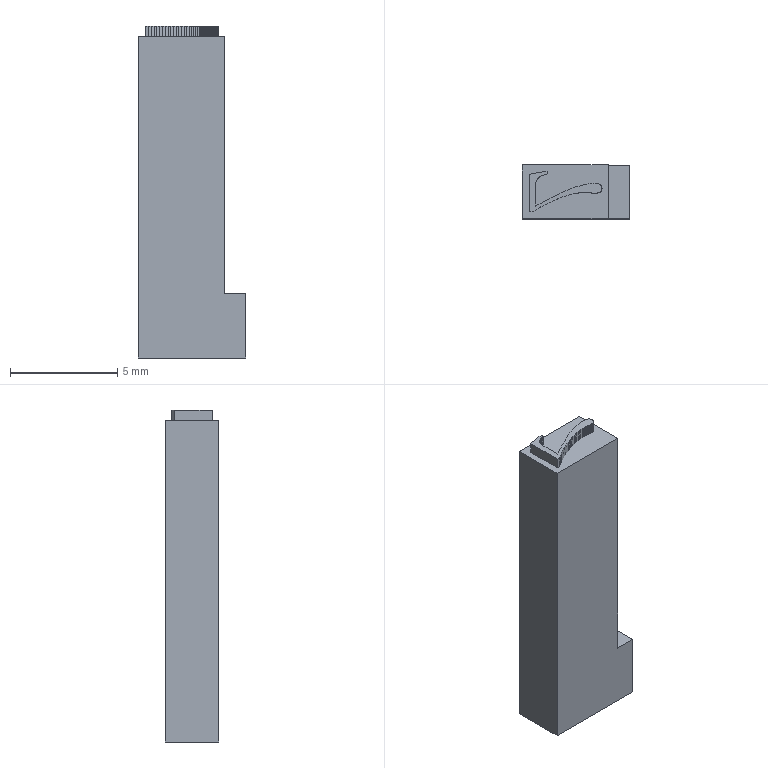Part | NX | features DIE-27 2 | 1 solid | 114 faces | box 5 x 2.5 x 15.5 mm | volume 158.247 mm3 | plane 114